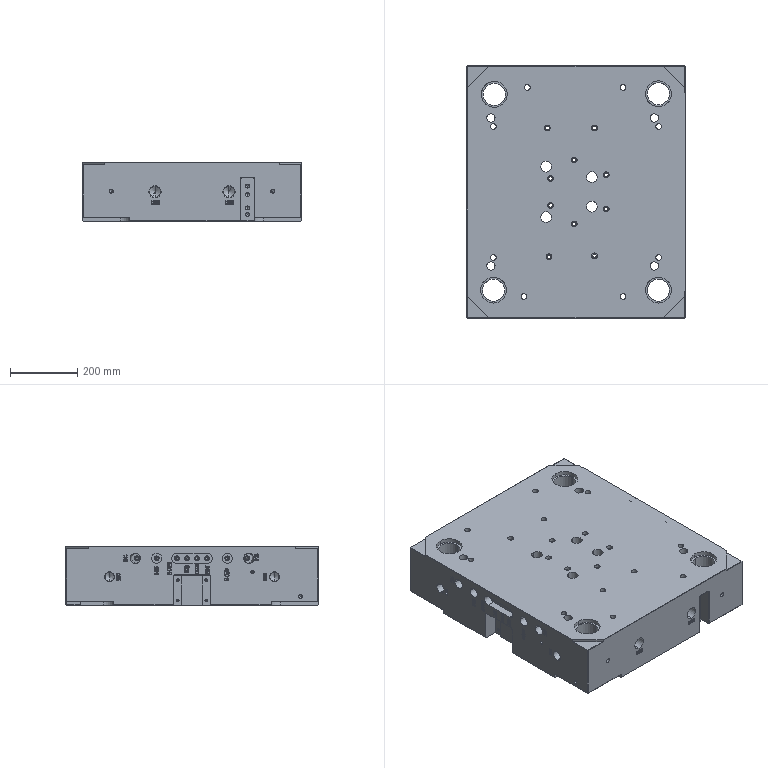Part | Creo | 1 solid | 3306 faces | volume 60537331 mm3 | plane 1250 | cylinder 949 | cone 536 | other 312 | torus 233 | spline 26 | commonest cylinder face diameters 10 x152 6 x96 5 x65 4.97 x64 19.1 x53 25.5 x53